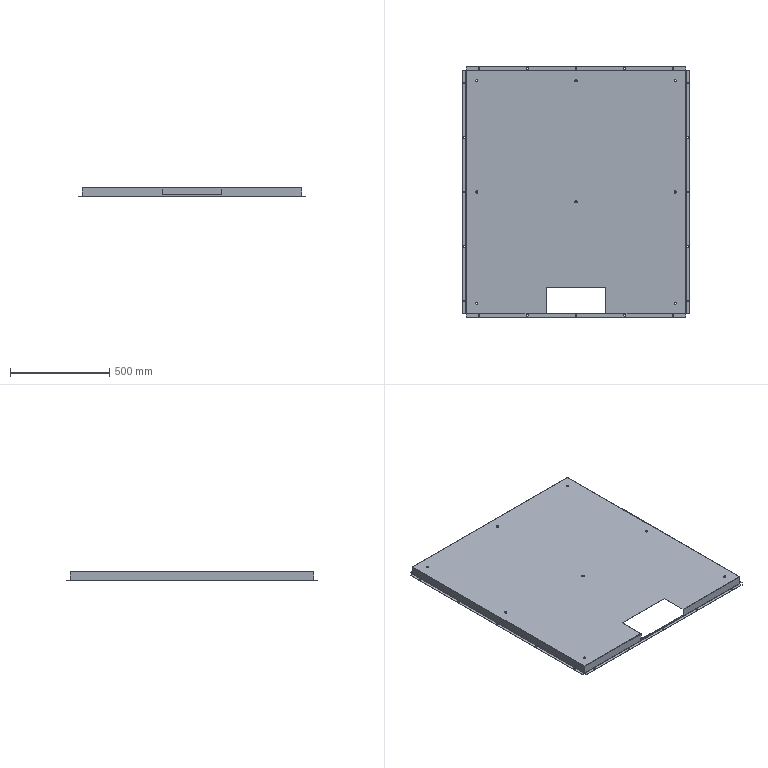Part | SolidWorks | features ICE 4, EdgeFlange 2, Cut 1, FlatPattern 1, SMBaseFlange 1, SheetMetal 1 | 1 solid | 186 faces | box 1140 x 1260 x 44 mm | volume 1579803 mm3 | plane 94 | cylinder 84 | spline 8 | commonest cylinder face diameters 7 x50 11 x16 1 x9 3 x9